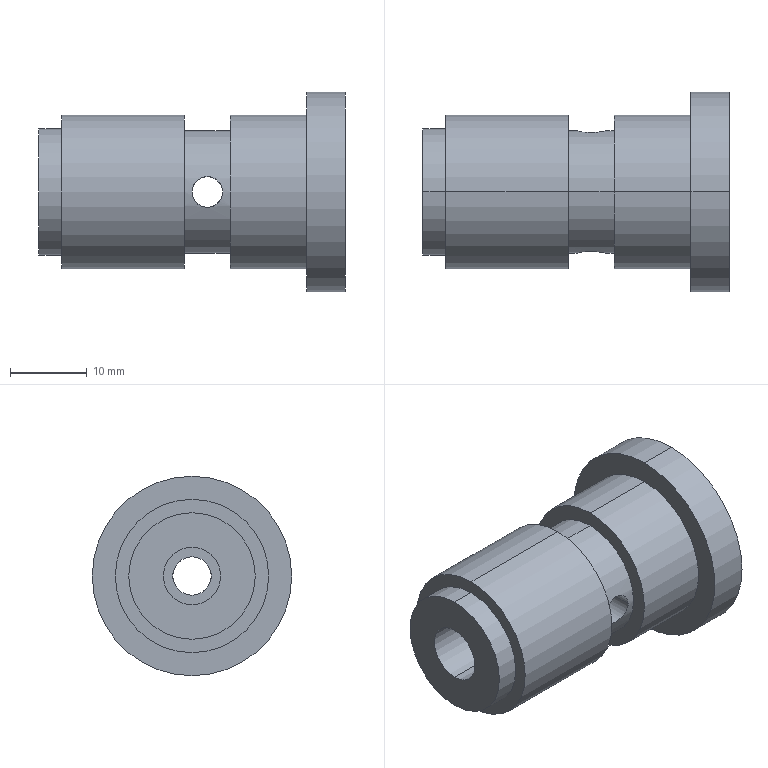Part | SolidWorks | features ICE 5, Cut 1, Extrusion 1, RevCut 1, SweepCut 1 | 1 solid | 34 faces | box 40 x 26 x 26 mm | volume 9972 mm3 | cylinder 24 | plane 10 | commonest cylinder face diameters 4 x4 16 x4 20 x4 5 x2 7.5 x2 14 x2
STEP:
#1=CARTESIAN_POINT('',(38.5,0.,-8.));
#2=VERTEX_POINT('',#1);
#3=CARTESIAN_POINT('',(38.5,0.,8.));
#4=VERTEX_POINT('',#3);
#5=CARTESIAN_POINT('',(38.5,0.,0.));
#6=DIRECTION('',(1.,0.,0.));
#7=DIRECTION('',(0.,0.,-1.));
#8=AXIS2_PLACEMENT_3D('',#5,#6,#7);
#9=CIRCLE('',#8,8.);
#10=EDGE_CURVE('',#2,#4,#9,.T.);
#11=ORIENTED_EDGE('',*,*,#10,.T.);
#12=CARTESIAN_POINT('',(40.,0.,8.));
#13=VERTEX_POINT('',#12);
#14=CARTESIAN_POINT('',(38.5,0.,8.));
#15=DIRECTION('',(1.,0.,0.));
#16=VECTOR('',#15,1000.);
#17=LINE('',#14,#16);
#18=EDGE_CURVE('',#4,#13,#17,.T.);
#19=ORIENTED_EDGE('',*,*,#18,.T.);
#20=CARTESIAN_POINT('',(40.,0.,-8.));
#21=VERTEX_POINT('',#20);
#22=CARTESIAN_POINT('',(40.,0.,0.));
#23=DIRECTION('',(1.,0.,0.));
#24=DIRECTION('',(0.,0.,-1.));
#25=AXIS2_PLACEMENT_3D('',#22,#23,#24);
#26=CIRCLE('',#25,8.);
#27=EDGE_CURVE('',#21,#13,#26,.T.);
#28=ORIENTED_EDGE('',*,*,#27,.F.);
#29=CARTESIAN_POINT('',(38.5,0.,-8.));
#30=DIRECTION('',(1.,0.,0.));
#31=VECTOR('',#30,1000.);
#32=LINE('',#29,#31);
#33=EDGE_CURVE('',#2,#21,#32,.T.);
#34=ORIENTED_EDGE('',*,*,#33,.F.);
#35=EDGE_LOOP('',(#11,#19,#28,#34));
#36=FACE_OUTER_BOUND('',#35,.T.);
#37=CARTESIAN_POINT('',(38.5,0.,0.));
#38=DIRECTION('',(1.,0.,0.));
#39=DIRECTION('',(0.,0.,-1.));
#40=AXIS2_PLACEMENT_3D('',#37,#38,#39);
#41=CYLINDRICAL_SURFACE('',#40,8.);
#42=ADVANCED_FACE('',(#36),#41,.T.);
#43=CARTESIAN_POINT('',(38.5,0.,11.));
#44=VERTEX_POINT('',#43);
#45=CARTESIAN_POINT('',(38.5,0.,-11.));
#46=VERTEX_POINT('',#45);
#47=CARTESIAN_POINT('',(38.5,0.,0.));
#48=DIRECTION('',(1.,0.,0.));
#49=DIRECTION('',(0.,0.,-1.));
#50=AXIS2_PLACEMENT_3D('',#47,#48,#49);
#51=CIRCLE('',#50,11.);
#52=EDGE_CURVE('',#44,#46,#51,.T.);
#53=ORIENTED_EDGE('',*,*,#52,.F.);
#54=CARTESIAN_POINT('',(40.,0.,11.));
#55=VERTEX_POINT('',#54);
#56=CARTESIAN_POINT('',(38.5,0.,11.));
#57=DIRECTION('',(1.,0.,0.));
#58=VECTOR('',#57,1000.);
#59=LINE('',#56,#58);
#60=EDGE_CURVE('',#44,#55,#59,.T.);
#61=ORIENTED_EDGE('',*,*,#60,.T.);
#62=CARTESIAN_POINT('',(40.,0.,-11.));
#63=VERTEX_POINT('',#62);
#64=CARTESIAN_POINT('',(40.,0.,0.));
#65=DIRECTION('',(1.,0.,0.));
#66=DIRECTION('',(0.,0.,-1.));
#67=AXIS2_PLACEMENT_3D('',#64,#65,#66);
#68=CIRCLE('',#67,11.);
#69=EDGE_CURVE('',#55,#63,#68,.T.);
#70=ORIENTED_EDGE('',*,*,#69,.T.);
#71=CARTESIAN_POINT('',(38.5,0.,-11.));
#72=DIRECTION('',(1.,0.,0.));
#73=VECTOR('',#72,1000.);
#74=LINE('',#71,#73);
#75=EDGE_CURVE('',#46,#63,#74,.T.);
#76=ORIENTED_EDGE('',*,*,#75,.F.);
#77=EDGE_LOOP('',(#53,#61,#70,#76));
#78=FACE_OUTER_BOUND('',#77,.T.);
#79=CARTESIAN_POINT('',(38.5,0.,0.));
#80=DIRECTION('',(1.,0.,0.));
#81=DIRECTION('',(0.,0.,-1.));
#82=AXIS2_PLACEMENT_3D('',#79,#80,#81);
#83=CYLINDRICAL_SURFACE('',#82,11.);
#84=ADVANCED_FACE('',(#78),#83,.F.);
#85=CARTESIAN_POINT('',(24.,8.,0.));
#86=VERTEX_POINT('',#85);
#87=CARTESIAN_POINT('',(20.,8.,0.));
#88=VERTEX_POINT('',#87);
#89=CARTESIAN_POINT('',(24.,8.,0.));
#90=CARTESIAN_POINT('',(24.,8.,-0.1327));
#91=CARTESIAN_POINT('',(23.987,7.997,-0.2631));
#92=CARTESIAN_POINT('',(23.936,7.984,-0.5195));
#93=CARTESIAN_POINT('',(23.897,7.975,-0.6468));
#94=CARTESIAN_POINT('',(23.796,7.951,-0.8888));
#95=CARTESIAN_POINT('',(23.735,7.938,-1.003));
#96=CARTESIAN_POINT('',(23.59,7.907,-1.22));
#97=CARTESIAN_POINT('',(23.506,7.89,-1.323));
#98=CARTESIAN_POINT('',(23.23,7.841,-1.598));
#99=CARTESIAN_POINT('',(23.008,7.808,-1.747));
#100=CARTESIAN_POINT('',(22.647,7.772,-1.897));
#101=CARTESIAN_POINT('',(22.52,7.762,-1.936));
#102=CARTESIAN_POINT('',(22.262,7.749,-1.987));
#103=CARTESIAN_POINT('',(22.132,7.746,-2.));
#104=CARTESIAN_POINT('',(21.87,7.746,-2.));
#105=CARTESIAN_POINT('',(21.737,7.749,-1.987));
#106=CARTESIAN_POINT('',(21.48,7.762,-1.936));
#107=CARTESIAN_POINT('',(21.355,7.772,-1.898));
#108=CARTESIAN_POINT('',(20.991,7.808,-1.746));
#109=CARTESIAN_POINT('',(20.771,7.841,-1.599));
#110=CARTESIAN_POINT('',(20.493,7.891,-1.321));
#111=CARTESIAN_POINT('',(20.41,7.907,-1.221));
#112=CARTESIAN_POINT('',(20.266,7.937,-1.005));
#113=CARTESIAN_POINT('',(20.203,7.952,-0.8874));
#114=CARTESIAN_POINT('',(20.103,7.975,-0.646));
#115=CARTESIAN_POINT('',(20.065,7.984,-0.5212));
#116=CARTESIAN_POINT('',(20.013,7.997,-0.2636));
#117=CARTESIAN_POINT('',(20.,8.,-0.1308));
#118=CARTESIAN_POINT('',(20.,8.,0.));
#119=B_SPLINE_CURVE_WITH_KNOTS('',3,(#89,#90,#91,#92,#93,#94,#95,#96,#97,#98,#99,#100,#101,#102,#103,#104,#105,#106,#107,#108,#109,#110,#111,#112,#113,#114,#115,#116,#117,#118),.UNSPECIFIED.,.F.,.F.,(4,2,2,2,2,2,2,2,2,2,2,2,2,2,4),(0.,0.0003924,0.0007847,0.001177,0.001569,0.002354,0.002747,0.003139,0.003531,0.003924,0.004708,0.005101,0.005493,0.005886,0.006278),.UNSPECIFIED.);
#120=EDGE_CURVE('',#86,#88,#119,.T.);
#121=ORIENTED_EDGE('',*,*,#120,.F.);
#122=CARTESIAN_POINT('',(20.,8.,0.));
#123=CARTESIAN_POINT('',(20.,8.,0.2616));
#124=CARTESIAN_POINT('',(20.053,7.986,0.5257));
#125=CARTESIAN_POINT('',(20.203,7.952,0.8871));
#126=CARTESIAN_POINT('',(20.265,7.937,1.004));
#127=CARTESIAN_POINT('',(20.411,7.907,1.221));
#128=CARTESIAN_POINT('',(20.493,7.891,1.321));
#129=CARTESIAN_POINT('',(20.677,7.858,1.506));
#130=CARTESIAN_POINT('',(20.78,7.841,1.59));
#131=CARTESIAN_POINT('',(20.996,7.81,1.734));
#132=CARTESIAN_POINT('',(21.11,7.796,1.796));
#133=CARTESIAN_POINT('',(21.475,7.76,1.948));
#134=CARTESIAN_POINT('',(21.736,7.746,2.));
#135=CARTESIAN_POINT('',(22.131,7.746,2.));
#136=CARTESIAN_POINT('',(22.261,7.749,1.987));
#137=CARTESIAN_POINT('',(22.518,7.762,1.936));
#138=CARTESIAN_POINT('',(22.646,7.772,1.897));
#139=CARTESIAN_POINT('',(23.008,7.808,1.747));
#140=CARTESIAN_POINT('',(23.23,7.841,1.598));
#141=CARTESIAN_POINT('',(23.597,7.907,1.232));
#142=CARTESIAN_POINT('',(23.746,7.94,1.01));
#143=CARTESIAN_POINT('',(23.896,7.975,0.6486));
#144=CARTESIAN_POINT('',(23.935,7.984,0.5212));
#145=CARTESIAN_POINT('',(23.987,7.997,0.2634));
#146=CARTESIAN_POINT('',(24.,8.,0.1327));
#147=CARTESIAN_POINT('',(24.,8.,0.));
#148=B_SPLINE_CURVE_WITH_KNOTS('',3,(#122,#123,#124,#125,#126,#127,#128,#129,#130,#131,#132,#133,#134,#135,#136,#137,#138,#139,#140,#141,#142,#143,#144,#145,#146,#147),.UNSPECIFIED.,.F.,.F.,(4,2,2,2,2,2,2,2,2,2,2,2,4),(0.006278,0.007062,0.007455,0.007847,0.008239,0.008631,0.009416,0.009808,0.0102,0.01099,0.01177,0.01216,0.01255),.UNSPECIFIED.);
#149=EDGE_CURVE('',#88,#86,#148,.T.);
#150=ORIENTED_EDGE('',*,*,#149,.F.);
#151=EDGE_LOOP('',(#121,#150));
#152=FACE_BOUND('',#151,.T.);
#153=CARTESIAN_POINT('',(19.,0.,-8.));
#154=VERTEX_POINT('',#153);
#155=CARTESIAN_POINT('',(19.,0.,8.));
#156=VERTEX_POINT('',#155);
#157=CARTESIAN_POINT('',(19.,0.,0.));
#158=DIRECTION('',(1.,0.,0.));
#159=DIRECTION('',(0.,0.,-1.));
#160=AXIS2_PLACEMENT_3D('',#157,#158,#159);
#161=CIRCLE('',#160,8.);
#162=EDGE_CURVE('',#154,#156,#161,.T.);
#163=ORIENTED_EDGE('',*,*,#162,.T.);
#164=CARTESIAN_POINT('',(25.,0.,8.));
#165=VERTEX_POINT('',#164);
#166=CARTESIAN_POINT('',(0.,0.,8.));
#167=DIRECTION('',(1.,0.,0.));
#168=VECTOR('',#167,1000.);
#169=LINE('',#166,#168);
#170=EDGE_CURVE('',#156,#165,#169,.T.);
#171=ORIENTED_EDGE('',*,*,#170,.T.);
#172=CARTESIAN_POINT('',(25.,0.,-8.));
#173=VERTEX_POINT('',#172);
#174=CARTESIAN_POINT('',(25.,0.,0.));
#175=DIRECTION('',(1.,0.,0.));
#176=DIRECTION('',(0.,0.,-1.));
#177=AXIS2_PLACEMENT_3D('',#174,#175,#176);
#178=CIRCLE('',#177,8.);
#179=EDGE_CURVE('',#173,#165,#178,.T.);
#180=ORIENTED_EDGE('',*,*,#179,.F.);
#181=CARTESIAN_POINT('',(0.,0.,-8.));
#182=DIRECTION('',(1.,0.,0.));
#183=VECTOR('',#182,1000.);
#184=LINE('',#181,#183);
#185=EDGE_CURVE('',#154,#173,#184,.T.);
#186=ORIENTED_EDGE('',*,*,#185,.F.);
#187=EDGE_LOOP('',(#163,#171,#180,#186));
#188=FACE_OUTER_BOUND('',#187,.T.);
#189=CARTESIAN_POINT('',(0.,0.,0.));
#190=DIRECTION('',(1.,0.,0.));
#191=DIRECTION('',(0.,0.,-1.));
#192=AXIS2_PLACEMENT_3D('',#189,#190,#191);
#193=CYLINDRICAL_SURFACE('',#192,8.);
#194=ADVANCED_FACE('',(#152,#188),#193,.T.);
#195=ORIENTED_EDGE('',*,*,#120,.T.);
#196=CARTESIAN_POINT('',(20.,2.5,0.));
#197=VERTEX_POINT('',#196);
#198=CARTESIAN_POINT('',(20.,11.268,0.));
#199=DIRECTION('',(0.,-1.,0.));
#200=VECTOR('',#199,1000.);
#201=LINE('',#198,#200);
#202=EDGE_CURVE('',#88,#197,#201,.T.);
#203=ORIENTED_EDGE('',*,*,#202,.T.);
#204=CARTESIAN_POINT('',(24.,2.5,0.));
#205=VERTEX_POINT('',#204);
#206=CARTESIAN_POINT('',(24.,2.5,0.));
#207=CARTESIAN_POINT('',(24.,2.5,-0.1403));
#208=CARTESIAN_POINT('',(23.985,2.488,-0.2771));
#209=CARTESIAN_POINT('',(23.929,2.444,-0.5445));
#210=CARTESIAN_POINT('',(23.887,2.41,-0.6754));
#211=CARTESIAN_POINT('',(23.782,2.329,-0.918));
#212=CARTESIAN_POINT('',(23.717,2.28,-1.033));
#213=CARTESIAN_POINT('',(23.572,2.172,-1.243));
#214=CARTESIAN_POINT('',(23.491,2.114,-1.339));
#215=CARTESIAN_POINT('',(23.314,1.993,-1.513));
#216=CARTESIAN_POINT('',(23.217,1.93,-1.592));
#217=CARTESIAN_POINT('',(23.01,1.807,-1.73));
#218=CARTESIAN_POINT('',(22.901,1.747,-1.79));
#219=CARTESIAN_POINT('',(22.668,1.639,-1.89));
#220=CARTESIAN_POINT('',(22.541,1.59,-1.93));
#221=CARTESIAN_POINT('',(22.278,1.52,-1.985));
#222=CARTESIAN_POINT('',(22.138,1.5,-2.));
#223=CARTESIAN_POINT('',(21.861,1.5,-2.));
#224=CARTESIAN_POINT('',(21.722,1.52,-1.985));
#225=CARTESIAN_POINT('',(21.458,1.59,-1.93));
#226=CARTESIAN_POINT('',(21.334,1.638,-1.89));
#227=CARTESIAN_POINT('',(20.979,1.802,-1.739));
#228=CARTESIAN_POINT('',(20.775,1.932,-1.601));
#229=CARTESIAN_POINT('',(20.508,2.115,-1.338));
#230=CARTESIAN_POINT('',(20.427,2.173,-1.242));
#231=CARTESIAN_POINT('',(20.283,2.279,-1.033));
#232=CARTESIAN_POINT('',(20.219,2.329,-0.9188));
#233=CARTESIAN_POINT('',(20.113,2.411,-0.6746));
#234=CARTESIAN_POINT('',(20.071,2.443,-0.5466));
#235=CARTESIAN_POINT('',(20.015,2.488,-0.2773));
#236=CARTESIAN_POINT('',(20.,2.5,-0.1381));
#237=CARTESIAN_POINT('',(20.,2.5,0.));
#238=B_SPLINE_CURVE_WITH_KNOTS('',3,(#206,#207,#208,#209,#210,#211,#212,#213,#214,#215,#216,#217,#218,#219,#220,#221,#222,#223,#224,#225,#226,#227,#228,#229,#230,#231,#232,#233,#234,#235,#236,#237),.UNSPECIFIED.,.F.,.F.,(4,2,2,2,2,2,2,2,2,2,2,2,2,2,2,4),(0.,0.0004139,0.0008279,0.001242,0.001656,0.00207,0.002484,0.002898,0.003311,0.003725,0.004139,0.004967,0.005381,0.005795,0.006209,0.006623),.UNSPECIFIED.);
#239=EDGE_CURVE('',#205,#197,#238,.T.);
#240=ORIENTED_EDGE('',*,*,#239,.F.);
#241=CARTESIAN_POINT('',(24.,11.268,0.));
#242=DIRECTION('',(0.,-1.,0.));
#243=VECTOR('',#242,1000.);
#244=LINE('',#241,#243);
#245=EDGE_CURVE('',#86,#205,#244,.T.);
#246=ORIENTED_EDGE('',*,*,#245,.F.);
#247=EDGE_LOOP('',(#195,#203,#240,#246));
#248=FACE_OUTER_BOUND('',#247,.T.);
#249=CARTESIAN_POINT('',(22.,11.268,0.));
#250=DIRECTION('',(0.,-1.,0.));
#251=DIRECTION('',(1.,0.,0.));
#252=AXIS2_PLACEMENT_3D('',#249,#250,#251);
#253=CYLINDRICAL_SURFACE('',#252,2.);
#254=ADVANCED_FACE('',(#248),#253,.F.);
#255=CARTESIAN_POINT('',(20.,-2.5,0.));
#256=VERTEX_POINT('',#255);
#257=CARTESIAN_POINT('',(24.,-2.5,0.));
#258=VERTEX_POINT('',#257);
#259=CARTESIAN_POINT('',(20.,-2.5,0.));
#260=CARTESIAN_POINT('',(20.,-2.5,-0.1377));
#261=CARTESIAN_POINT('',(20.015,-2.488,-0.2778));
#262=CARTESIAN_POINT('',(20.071,-2.444,-0.545));
#263=CARTESIAN_POINT('',(20.112,-2.411,-0.6743));
#264=CARTESIAN_POINT('',(20.271,-2.288,-1.04));
#265=CARTESIAN_POINT('',(20.421,-2.174,-1.252));
#266=CARTESIAN_POINT('',(20.775,-1.932,-1.6));
#267=CARTESIAN_POINT('',(20.982,-1.801,-1.74));
#268=CARTESIAN_POINT('',(21.331,-1.639,-1.889));
#269=CARTESIAN_POINT('',(21.456,-1.59,-1.929));
#270=CARTESIAN_POINT('',(21.72,-1.521,-1.985));
#271=CARTESIAN_POINT('',(21.859,-1.5,-2.));
#272=CARTESIAN_POINT('',(22.138,-1.5,-2.));
#273=CARTESIAN_POINT('',(22.276,-1.52,-1.986));
#274=CARTESIAN_POINT('',(22.541,-1.589,-1.93));
#275=CARTESIAN_POINT('',(22.664,-1.637,-1.891));
#276=CARTESIAN_POINT('',(22.9,-1.746,-1.791));
#277=CARTESIAN_POINT('',(23.011,-1.807,-1.73));
#278=CARTESIAN_POINT('',(23.216,-1.929,-1.593));
#279=CARTESIAN_POINT('',(23.312,-1.992,-1.515));
#280=CARTESIAN_POINT('',(23.49,-2.114,-1.34));
#281=CARTESIAN_POINT('',(23.572,-2.172,-1.243));
#282=CARTESIAN_POINT('',(23.716,-2.279,-1.034));
#283=CARTESIAN_POINT('',(23.78,-2.327,-0.9222));
#284=CARTESIAN_POINT('',(23.886,-2.41,-0.6783));
#285=CARTESIAN_POINT('',(23.928,-2.443,-0.5484));
#286=CARTESIAN_POINT('',(23.985,-2.488,-0.2808));
#287=CARTESIAN_POINT('',(24.,-2.5,-0.1398));
#288=CARTESIAN_POINT('',(24.,-2.5,0.));
#289=B_SPLINE_CURVE_WITH_KNOTS('',3,(#259,#260,#261,#262,#263,#264,#265,#266,#267,#268,#269,#270,#271,#272,#273,#274,#275,#276,#277,#278,#279,#280,#281,#282,#283,#284,#285,#286,#287,#288),.UNSPECIFIED.,.F.,.F.,(4,2,2,2,2,2,2,2,2,2,2,2,2,2,4),(0.006623,0.007035,0.007448,0.008273,0.009098,0.009511,0.009924,0.01034,0.01075,0.01116,0.01157,0.01199,0.0124,0.01281,0.01322),.UNSPECIFIED.);
#290=EDGE_CURVE('',#256,#258,#289,.T.);
#291=ORIENTED_EDGE('',*,*,#290,.F.);
#292=CARTESIAN_POINT('',(20.,-8.,0.));
#293=VERTEX_POINT('',#292);
#294=CARTESIAN_POINT('',(20.,11.268,0.));
#295=DIRECTION('',(0.,-1.,0.));
#296=VECTOR('',#295,1000.);
#297=LINE('',#294,#296);
#298=EDGE_CURVE('',#256,#293,#297,.T.);
#299=ORIENTED_EDGE('',*,*,#298,.T.);
#300=CARTESIAN_POINT('',(24.,-8.,0.));
#301=VERTEX_POINT('',#300);
#302=CARTESIAN_POINT('',(20.,-8.,0.));
#303=CARTESIAN_POINT('',(20.,-8.,-0.2616));
#304=CARTESIAN_POINT('',(20.053,-7.986,-0.5257));
#305=CARTESIAN_POINT('',(20.203,-7.952,-0.8871));
#306=CARTESIAN_POINT('',(20.265,-7.937,-1.004));
#307=CARTESIAN_POINT('',(20.411,-7.907,-1.221));
#308=CARTESIAN_POINT('',(20.493,-7.891,-1.321));
#309=CARTESIAN_POINT('',(20.677,-7.858,-1.506));
#310=CARTESIAN_POINT('',(20.78,-7.841,-1.59));
#311=CARTESIAN_POINT('',(20.996,-7.81,-1.734));
#312=CARTESIAN_POINT('',(21.11,-7.796,-1.796));
#313=CARTESIAN_POINT('',(21.475,-7.76,-1.948));
#314=CARTESIAN_POINT('',(21.736,-7.746,-2.));
#315=CARTESIAN_POINT('',(22.131,-7.746,-2.));
#316=CARTESIAN_POINT('',(22.261,-7.749,-1.987));
#317=CARTESIAN_POINT('',(22.518,-7.762,-1.936));
#318=CARTESIAN_POINT('',(22.646,-7.772,-1.897));
#319=CARTESIAN_POINT('',(23.008,-7.808,-1.747));
#320=CARTESIAN_POINT('',(23.23,-7.841,-1.598));
#321=CARTESIAN_POINT('',(23.597,-7.907,-1.232));
#322=CARTESIAN_POINT('',(23.746,-7.94,-1.01));
#323=CARTESIAN_POINT('',(23.896,-7.975,-0.6486));
#324=CARTESIAN_POINT('',(23.935,-7.984,-0.5212));
#325=CARTESIAN_POINT('',(23.987,-7.997,-0.2634));
#326=CARTESIAN_POINT('',(24.,-8.,-0.1327));
#327=CARTESIAN_POINT('',(24.,-8.,0.));
#328=B_SPLINE_CURVE_WITH_KNOTS('',3,(#302,#303,#304,#305,#306,#307,#308,#309,#310,#311,#312,#313,#314,#315,#316,#317,#318,#319,#320,#321,#322,#323,#324,#325,#326,#327),.UNSPECIFIED.,.F.,.F.,(4,2,2,2,2,2,2,2,2,2,2,2,4),(0.006278,0.007062,0.007455,0.007847,0.008239,0.008631,0.009416,0.009808,0.0102,0.01099,0.01177,0.01216,0.01255),.UNSPECIFIED.);
#329=EDGE_CURVE('',#293,#301,#328,.T.);
#330=ORIENTED_EDGE('',*,*,#329,.T.);
#331=CARTESIAN_POINT('',(24.,11.268,0.));
#332=DIRECTION('',(0.,-1.,0.));
#333=VECTOR('',#332,1000.);
#334=LINE('',#331,#333);
#335=EDGE_CURVE('',#258,#301,#334,.T.);
#336=ORIENTED_EDGE('',*,*,#335,.F.);
#337=EDGE_LOOP('',(#291,#299,#330,#336));
#338=FACE_OUTER_BOUND('',#337,.T.);
#339=CARTESIAN_POINT('',(22.,11.268,0.));
#340=DIRECTION('',(0.,-1.,0.));
#341=DIRECTION('',(1.,0.,0.));
#342=AXIS2_PLACEMENT_3D('',#339,#340,#341);
#343=CYLINDRICAL_SURFACE('',#342,2.);
#344=ADVANCED_FACE('',(#338),#343,.F.);
#345=CARTESIAN_POINT('',(6.5,0.,-3.75));
#346=VERTEX_POINT('',#345);
#347=CARTESIAN_POINT('',(6.5,0.,3.75));
#348=VERTEX_POINT('',#347);
#349=CARTESIAN_POINT('',(6.5,0.,0.));
#350=DIRECTION('',(-1.,0.,0.));
#351=DIRECTION('',(0.,0.,1.));
#352=AXIS2_PLACEMENT_3D('',#349,#350,#351);
#353=CIRCLE('',#352,3.75);
#354=EDGE_CURVE('',#346,#348,#353,.T.);
#355=ORIENTED_EDGE('',*,*,#354,.F.);
#356=CARTESIAN_POINT('',(0.,0.,-3.75));
#357=VERTEX_POINT('',#356);
#358=CARTESIAN_POINT('',(6.5,0.,-3.75));
#359=DIRECTION('',(-1.,0.,0.));
#360=VECTOR('',#359,1000.);
#361=LINE('',#358,#360);
#362=EDGE_CURVE('',#346,#357,#361,.T.);
#363=ORIENTED_EDGE('',*,*,#362,.T.);
#364=CARTESIAN_POINT('',(0.,0.,3.75));
#365=VERTEX_POINT('',#364);
#366=CARTESIAN_POINT('',(0.,0.,0.));
#367=DIRECTION('',(-1.,0.,0.));
#368=DIRECTION('',(0.,0.,1.));
#369=AXIS2_PLACEMENT_3D('',#366,#367,#368);
#370=CIRCLE('',#369,3.75);
#371=EDGE_CURVE('',#357,#365,#370,.T.);
#372=ORIENTED_EDGE('',*,*,#371,.T.);
#373=CARTESIAN_POINT('',(6.5,0.,3.75));
#374=DIRECTION('',(-1.,0.,0.));
#375=VECTOR('',#374,1000.);
#376=LINE('',#373,#375);
#377=EDGE_CURVE('',#348,#365,#376,.T.);
#378=ORIENTED_EDGE('',*,*,#377,.F.);
#379=EDGE_LOOP('',(#355,#363,#372,#378));
#380=FACE_OUTER_BOUND('',#379,.T.);
#381=CARTESIAN_POINT('',(6.5,0.,0.));
#382=DIRECTION('',(-1.,0.,0.));
#383=DIRECTION('',(0.,0.,1.));
#384=AXIS2_PLACEMENT_3D('',#381,#382,#383);
#385=CYLINDRICAL_SURFACE('',#384,3.75);
#386=ADVANCED_FACE('',(#380),#385,.F.);
#387=CARTESIAN_POINT('',(30.,0.,7.));
#388=VERTEX_POINT('',#387);
#389=CARTESIAN_POINT('',(30.,0.,-7.));
#390=VERTEX_POINT('',#389);
#391=CARTESIAN_POINT('',(30.,0.,0.));
#392=DIRECTION('',(1.,0.,0.));
#393=DIRECTION('',(0.,0.,-1.));
#394=AXIS2_PLACEMENT_3D('',#391,#392,#393);
#395=CIRCLE('',#394,7.);
#396=EDGE_CURVE('',#388,#390,#395,.T.);
#397=ORIENTED_EDGE('',*,*,#396,.F.);
#398=CARTESIAN_POINT('',(40.,0.,7.));
#399=VERTEX_POINT('',#398);
#400=CARTESIAN_POINT('',(30.,0.,7.));
#401=DIRECTION('',(1.,0.,0.));
#402=VECTOR('',#401,1000.);
#403=LINE('',#400,#402);
#404=EDGE_CURVE('',#388,#399,#403,.T.);
#405=ORIENTED_EDGE('',*,*,#404,.T.);
#406=CARTESIAN_POINT('',(40.,0.,-7.));
#407=VERTEX_POINT('',#406);
#408=CARTESIAN_POINT('',(40.,0.,0.));
#409=DIRECTION('',(1.,0.,0.));
#410=DIRECTION('',(0.,0.,-1.));
#411=AXIS2_PLACEMENT_3D('',#408,#409,#410);
#412=CIRCLE('',#411,7.);
#413=EDGE_CURVE('',#399,#407,#412,.T.);
#414=ORIENTED_EDGE('',*,*,#413,.T.);
#415=CARTESIAN_POINT('',(30.,0.,-7.));
#416=DIRECTION('',(1.,0.,0.));
#417=VECTOR('',#416,1000.);
#418=LINE('',#415,#417);
#419=EDGE_CURVE('',#390,#407,#418,.T.);
#420=ORIENTED_EDGE('',*,*,#419,.F.);
#421=EDGE_LOOP('',(#397,#405,#414,#420));
#422=FACE_OUTER_BOUND('',#421,.T.);
#423=CARTESIAN_POINT('',(30.,0.,0.));
#424=DIRECTION('',(1.,0.,0.));
#425=DIRECTION('',(0.,0.,-1.));
#426=AXIS2_PLACEMENT_3D('',#423,#424,#425);
#427=CYLINDRICAL_SURFACE('',#426,7.);
#428=ADVANCED_FACE('',(#422),#427,.F.);
#429=CARTESIAN_POINT('',(40.,0.,-13.));
#430=VERTEX_POINT('',#429);
#431=CARTESIAN_POINT('',(40.,0.,13.));
#432=VERTEX_POINT('',#431);
#433=CARTESIAN_POINT('',(40.,0.,0.));
#434=DIRECTION('',(1.,0.,0.));
#435=DIRECTION('',(0.,0.,-1.));
#436=AXIS2_PLACEMENT_3D('',#433,#434,#435);
#437=CIRCLE('',#436,13.);
#438=EDGE_CURVE('',#430,#432,#437,.T.);
#439=ORIENTED_EDGE('',*,*,#438,.F.);
#440=CARTESIAN_POINT('',(35.,0.,-13.));
#441=VERTEX_POINT('',#440);
#442=CARTESIAN_POINT('',(40.,0.,-13.));
#443=DIRECTION('',(-1.,0.,0.));
#444=VECTOR('',#443,1000.);
#445=LINE('',#442,#444);
#446=EDGE_CURVE('',#430,#441,#445,.T.);
#447=ORIENTED_EDGE('',*,*,#446,.T.);
#448=CARTESIAN_POINT('',(35.,0.,13.));
#449=VERTEX_POINT('',#448);
#450=CARTESIAN_POINT('',(35.,0.,0.));
#451=DIRECTION('',(1.,0.,0.));
#452=DIRECTION('',(0.,0.,-1.));
#453=AXIS2_PLACEMENT_3D('',#450,#451,#452);
#454=CIRCLE('',#453,13.);
#455=EDGE_CURVE('',#441,#449,#454,.T.);
#456=ORIENTED_EDGE('',*,*,#455,.T.);
#457=CARTESIAN_POINT('',(40.,0.,13.));
#458=DIRECTION('',(-1.,0.,0.));
#459=VECTOR('',#458,1000.);
#460=LINE('',#457,#459);
#461=EDGE_CURVE('',#432,#449,#460,.T.);
#462=ORIENTED_EDGE('',*,*,#461,.F.);
#463=EDGE_LOOP('',(#439,#447,#456,#462));
#464=FACE_OUTER_BOUND('',#463,.T.);
#465=CARTESIAN_POINT('',(40.,0.,0.));
#466=DIRECTION('',(-1.,0.,0.));
#467=DIRECTION('',(0.,0.,1.));
#468=AXIS2_PLACEMENT_3D('',#465,#466,#467);
#469=CYLINDRICAL_SURFACE('',#468,13.);
#470=ADVANCED_FACE('',(#464),#469,.T.);
#471=CARTESIAN_POINT('',(19.,0.,10.));
#472=VERTEX_POINT('',#471);
#473=CARTESIAN_POINT('',(19.,0.,-10.));
#474=VERTEX_POINT('',#473);
#475=CARTESIAN_POINT('',(19.,0.,0.));
#476=DIRECTION('',(-1.,0.,0.));
#477=DIRECTION('',(0.,0.,1.));
#478=AXIS2_PLACEMENT_3D('',#475,#476,#477);
#479=CIRCLE('',#478,10.);
#480=EDGE_CURVE('',#472,#474,#479,.T.);
#481=ORIENTED_EDGE('',*,*,#480,.T.);
#482=CARTESIAN_POINT('',(3.,0.,-10.));
#483=VERTEX_POINT('',#482);
#484=CARTESIAN_POINT('',(35.,0.,-10.));
#485=DIRECTION('',(-1.,0.,0.));
#486=VECTOR('',#485,1000.);
#487=LINE('',#484,#486);
#488=EDGE_CURVE('',#474,#483,#487,.T.);
#489=ORIENTED_EDGE('',*,*,#488,.T.);
#490=CARTESIAN_POINT('',(3.,0.,10.));
#491=VERTEX_POINT('',#490);
#492=CARTESIAN_POINT('',(3.,0.,0.));
#493=DIRECTION('',(1.,0.,0.));
#494=DIRECTION('',(0.,0.,-1.));
#495=AXIS2_PLACEMENT_3D('',#492,#493,#494);
#496=CIRCLE('',#495,10.);
#497=EDGE_CURVE('',#483,#491,#496,.T.);
#498=ORIENTED_EDGE('',*,*,#497,.T.);
#499=CARTESIAN_POINT('',(35.,0.,10.));
#500=DIRECTION('',(-1.,0.,0.));
#501=VECTOR('',#500,1000.);
#502=LINE('',#499,#501);
#503=EDGE_CURVE('',#472,#491,#502,.T.);
#504=ORIENTED_EDGE('',*,*,#503,.F.);
#505=EDGE_LOOP('',(#481,#489,#498,#504));
#506=FACE_OUTER_BOUND('',#505,.T.);
#507=CARTESIAN_POINT('',(35.,0.,0.));
#508=DIRECTION('',(-1.,0.,0.));
#509=DIRECTION('',(0.,0.,1.));
#510=AXIS2_PLACEMENT_3D('',#507,#508,#509);
#511=CYLINDRICAL_SURFACE('',#510,10.);
#512=ADVANCED_FACE('',(#506),#511,.T.);
#513=CARTESIAN_POINT('',(3.,0.,-8.25));
#514=VERTEX_POINT('',#513);
#515=CARTESIAN_POINT('',(3.,0.,8.25));
#516=VERTEX_POINT('',#515);
#517=CARTESIAN_POINT('',(3.,0.,0.));
#518=DIRECTION('',(1.,0.,0.));
#519=DIRECTION('',(0.,0.,-1.));
#520=AXIS2_PLACEMENT_3D('',#517,#518,#519);
#521=CIRCLE('',#520,8.25);
#522=EDGE_CURVE('',#514,#516,#521,.T.);
#523=ORIENTED_EDGE('',*,*,#522,.F.);
#524=CARTESIAN_POINT('',(0.,0.,-8.25));
#525=VERTEX_POINT('',#524);
#526=CARTESIAN_POINT('',(3.,0.,-8.25));
#527=DIRECTION('',(-1.,0.,0.));
#528=VECTOR('',#527,1000.);
#529=LINE('',#526,#528);
#530=EDGE_CURVE('',#514,#525,#529,.T.);
#531=ORIENTED_EDGE('',*,*,#530,.T.);
#532=CARTESIAN_POINT('',(0.,0.,8.25));
#533=VERTEX_POINT('',#532);
#534=CARTESIAN_POINT('',(0.,0.,0.));
#535=DIRECTION('',(1.,0.,0.));
#536=DIRECTION('',(0.,0.,-1.));
#537=AXIS2_PLACEMENT_3D('',#534,#535,#536);
#538=CIRCLE('',#537,8.25);
#539=EDGE_CURVE('',#525,#533,#538,.T.);
#540=ORIENTED_EDGE('',*,*,#539,.T.);
#541=CARTESIAN_POINT('',(3.,0.,8.25));
#542=DIRECTION('',(-1.,0.,0.));
#543=VECTOR('',#542,1000.);
#544=LINE('',#541,#543);
#545=EDGE_CURVE('',#516,#533,#544,.T.);
#546=ORIENTED_EDGE('',*,*,#545,.F.);
#547=EDGE_LOOP('',(#523,#531,#540,#546));
#548=FACE_OUTER_BOUND('',#547,.T.);
#549=CARTESIAN_POINT('',(3.,0.,0.));
#550=DIRECTION('',(-1.,0.,0.));
#551=DIRECTION('',(0.,0.,1.));
#552=AXIS2_PLACEMENT_3D('',#549,#550,#551);
#553=CYLINDRICAL_SURFACE('',#552,8.25);
#554=ADVANCED_FACE('',(#548),#553,.T.);
#555=CARTESIAN_POINT('',(24.,-2.5,0.));
#556=CARTESIAN_POINT('',(24.,-2.5,0.1403));
#557=CARTESIAN_POINT('',(23.985,-2.488,0.2771));
#558=CARTESIAN_POINT('',(23.929,-2.444,0.5445));
#559=CARTESIAN_POINT('',(23.887,-2.41,0.6754));
#560=CARTESIAN_POINT('',(23.782,-2.329,0.918));
#561=CARTESIAN_POINT('',(23.717,-2.28,1.033));
#562=CARTESIAN_POINT('',(23.572,-2.172,1.243));
#563=CARTESIAN_POINT('',(23.491,-2.114,1.339));
#564=CARTESIAN_POINT('',(23.314,-1.993,1.513));
#565=CARTESIAN_POINT('',(23.217,-1.93,1.592));
#566=CARTESIAN_POINT('',(23.01,-1.807,1.73));
#567=CARTESIAN_POINT('',(22.901,-1.747,1.79));
#568=CARTESIAN_POINT('',(22.668,-1.639,1.89));
#569=CARTESIAN_POINT('',(22.541,-1.59,1.93));
#570=CARTESIAN_POINT('',(22.278,-1.52,1.985));
#571=CARTESIAN_POINT('',(22.138,-1.5,2.));
#572=CARTESIAN_POINT('',(21.861,-1.5,2.));
#573=CARTESIAN_POINT('',(21.722,-1.52,1.985));
#574=CARTESIAN_POINT('',(21.458,-1.59,1.93));
#575=CARTESIAN_POINT('',(21.334,-1.638,1.89));
#576=CARTESIAN_POINT('',(20.979,-1.802,1.739));
#577=CARTESIAN_POINT('',(20.775,-1.932,1.601));
#578=CARTESIAN_POINT('',(20.508,-2.115,1.338));
#579=CARTESIAN_POINT('',(20.427,-2.173,1.242));
#580=CARTESIAN_POINT('',(20.283,-2.279,1.033));
#581=CARTESIAN_POINT('',(20.219,-2.329,0.9188));
#582=CARTESIAN_POINT('',(20.113,-2.411,0.6746));
#583=CARTESIAN_POINT('',(20.071,-2.443,0.5466));
#584=CARTESIAN_POINT('',(20.015,-2.488,0.2773));
#585=CARTESIAN_POINT('',(20.,-2.5,0.1381));
#586=CARTESIAN_POINT('',(20.,-2.5,0.));
#587=B_SPLINE_CURVE_WITH_KNOTS('',3,(#555,#556,#557,#558,#559,#560,#561,#562,#563,#564,#565,#566,#567,#568,#569,#570,#571,#572,#573,#574,#575,#576,#577,#578,#579,#580,#581,#582,#583,#584,#585,#586),.UNSPECIFIED.,.F.,.F.,(4,2,2,2,2,2,2,2,2,2,2,2,2,2,2,4),(0.,0.0004139,0.0008279,0.001242,0.001656,0.00207,0.002484,0.002898,0.003311,0.003725,0.004139,0.004967,0.005381,0.005795,0.006209,0.006623),.UNSPECIFIED.);
#588=EDGE_CURVE('',#258,#256,#587,.T.);
#589=ORIENTED_EDGE('',*,*,#588,.T.);
#590=ORIENTED_EDGE('',*,*,#290,.T.);
#591=EDGE_LOOP('',(#589,#590));
#592=FACE_BOUND('',#591,.T.);
#593=CARTESIAN_POINT('',(6.5,0.,2.5));
#594=VERTEX_POINT('',#593);
#595=CARTESIAN_POINT('',(6.5,0.,-2.5));
#596=VERTEX_POINT('',#595);
#597=CARTESIAN_POINT('',(6.5,0.,0.));
#598=DIRECTION('',(1.,0.,0.));
#599=DIRECTION('',(0.,0.,1.));
#600=AXIS2_PLACEMENT_3D('',#597,#598,#599);
#601=CIRCLE('',#600,2.5);
#602=EDGE_CURVE('',#594,#596,#601,.T.);
#603=ORIENTED_EDGE('',*,*,#602,.F.);
#604=CARTESIAN_POINT('',(30.,0.,2.5));
#605=VERTEX_POINT('',#604);
#606=CARTESIAN_POINT('',(-3.,0.,2.5));
#607=DIRECTION('',(1.,0.,0.));
#608=VECTOR('',#607,1000.);
#609=LINE('',#606,#608);
#610=EDGE_CURVE('',#594,#605,#609,.T.);
#611=ORIENTED_EDGE('',*,*,#610,.T.);
#612=CARTESIAN_POINT('',(30.,0.,-2.5));
#613=VERTEX_POINT('',#612);
#614=CARTESIAN_POINT('',(30.,0.,0.));
#615=DIRECTION('',(1.,0.,0.));
#616=DIRECTION('',(0.,0.,-1.));
#617=AXIS2_PLACEMENT_3D('',#614,#615,#616);
#618=CIRCLE('',#617,2.5);
#619=EDGE_CURVE('',#605,#613,#618,.T.);
#620=ORIENTED_EDGE('',*,*,#619,.T.);
#621=CARTESIAN_POINT('',(-3.,0.,-2.5));
#622=DIRECTION('',(1.,0.,0.));
#623=VECTOR('',#622,1000.);
#624=LINE('',#621,#623);
#625=EDGE_CURVE('',#596,#613,#624,.T.);
#626=ORIENTED_EDGE('',*,*,#625,.F.);
#627=EDGE_LOOP('',(#603,#611,#620,#626));
#628=FACE_OUTER_BOUND('',#627,.T.);
#629=CARTESIAN_POINT('',(-3.,0.,0.));
#630=DIRECTION('',(1.,0.,0.));
#631=DIRECTION('',(0.,0.,-1.));
#632=AXIS2_PLACEMENT_3D('',#629,#630,#631);
#633=CYLINDRICAL_SURFACE('',#632,2.5);
#634=ADVANCED_FACE('',(#592,#628),#633,.F.);
#635=CARTESIAN_POINT('',(35.,0.,-10.));
#636=VERTEX_POINT('',#635);
#637=CARTESIAN_POINT('',(35.,0.,10.));
#638=VERTEX_POINT('',#637);
#639=CARTESIAN_POINT('',(35.,0.,0.));
#640=DIRECTION('',(1.,0.,0.));
#641=DIRECTION('',(0.,0.,-1.));
#642=AXIS2_PLACEMENT_3D('',#639,#640,#641);
#643=CIRCLE('',#642,10.);
#644=EDGE_CURVE('',#636,#638,#643,.T.);
#645=ORIENTED_EDGE('',*,*,#644,.F.);
#646=CARTESIAN_POINT('',(25.,0.,-10.));
#647=VERTEX_POINT('',#646);
#648=CARTESIAN_POINT('',(35.,0.,-10.));
#649=DIRECTION('',(-1.,0.,0.));
#650=VECTOR('',#649,1000.);
#651=LINE('',#648,#650);
#652=EDGE_CURVE('',#636,#647,#651,.T.);
#653=ORIENTED_EDGE('',*,*,#652,.T.);
#654=CARTESIAN_POINT('',(25.,0.,10.));
#655=VERTEX_POINT('',#654);
#656=CARTESIAN_POINT('',(25.,0.,0.));
#657=DIRECTION('',(1.,0.,0.));
#658=DIRECTION('',(0.,0.,-1.));
#659=AXIS2_PLACEMENT_3D('',#656,#657,#658);
#660=CIRCLE('',#659,10.);
#661=EDGE_CURVE('',#647,#655,#660,.T.);
#662=ORIENTED_EDGE('',*,*,#661,.T.);
#663=CARTESIAN_POINT('',(35.,0.,10.));
#664=DIRECTION('',(-1.,0.,0.));
#665=VECTOR('',#664,1000.);
#666=LINE('',#663,#665);
#667=EDGE_CURVE('',#638,#655,#666,.T.);
#668=ORIENTED_EDGE('',*,*,#667,.F.);
#669=EDGE_LOOP('',(#645,#653,#662,#668));
#670=FACE_OUTER_BOUND('',#669,.T.);
#671=CARTESIAN_POINT('',(35.,0.,0.));
#672=DIRECTION('',(-1.,0.,0.));
#673=DIRECTION('',(0.,0.,1.));
#674=AXIS2_PLACEMENT_3D('',#671,#672,#673);
#675=CYLINDRICAL_SURFACE('',#674,10.);
#676=ADVANCED_FACE('',(#670),#675,.T.);
#677=CARTESIAN_POINT('',(40.,0.,0.));
#678=DIRECTION('',(1.,0.,0.));
#679=DIRECTION('',(0.,0.,-1.));
#680=AXIS2_PLACEMENT_3D('',#677,#678,#679);
#681=CIRCLE('',#680,7.);
#682=EDGE_CURVE('',#407,#399,#681,.T.);
#683=ORIENTED_EDGE('',*,*,#682,.F.);
#684=ORIENTED_EDGE('',*,*,#413,.F.);
#685=EDGE_LOOP('',(#683,#684));
#686=FACE_BOUND('',#685,.T.);
#687=ORIENTED_EDGE('',*,*,#27,.T.);
#688=CARTESIAN_POINT('',(40.,0.,0.));
#689=DIRECTION('',(1.,0.,0.));
#690=DIRECTION('',(0.,0.,-1.));
#691=AXIS2_PLACEMENT_3D('',#688,#689,#690);
#692=CIRCLE('',#691,8.);
#693=EDGE_CURVE('',#13,#21,#692,.T.);
#694=ORIENTED_EDGE('',*,*,#693,.T.);
#695=EDGE_LOOP('',(#687,#694));
#696=FACE_OUTER_BOUND('',#695,.T.);
#697=CARTESIAN_POINT('',(40.,0.,0.));
#698=DIRECTION('',(1.,0.,0.));
#699=DIRECTION('',(0.,0.,-1.));
#700=AXIS2_PLACEMENT_3D('',#697,#698,#699);
#701=PLANE('',#700);
#702=ADVANCED_FACE('',(#686,#696),#701,.T.);
#703=ORIENTED_EDGE('',*,*,#652,.F.);
#704=CARTESIAN_POINT('',(35.,0.,0.));
#705=DIRECTION('',(1.,0.,0.));
#706=DIRECTION('',(0.,0.,-1.));
#707=AXIS2_PLACEMENT_3D('',#704,#705,#706);
#708=CIRCLE('',#707,10.);
#709=EDGE_CURVE('',#638,#636,#708,.T.);
#710=ORIENTED_EDGE('',*,*,#709,.F.);
#711=ORIENTED_EDGE('',*,*,#667,.T.);
#712=CARTESIAN_POINT('',(25.,0.,0.));
#713=DIRECTION('',(1.,0.,0.));
#714=DIRECTION('',(0.,0.,-1.));
#715=AXIS2_PLACEMENT_3D('',#712,#713,#714);
#716=CIRCLE('',#715,10.);
#717=EDGE_CURVE('',#655,#647,#716,.T.);
#718=ORIENTED_EDGE('',*,*,#717,.T.);
#719=EDGE_LOOP('',(#703,#710,#711,#718));
#720=FACE_OUTER_BOUND('',#719,.T.);
#721=CARTESIAN_POINT('',(35.,0.,0.));
#722=DIRECTION('',(-1.,0.,0.));
#723=DIRECTION('',(0.,0.,1.));
#724=AXIS2_PLACEMENT_3D('',#721,#722,#723);
#725=CYLINDRICAL_SURFACE('',#724,10.);
#726=ADVANCED_FACE('',(#720),#725,.T.);
#727=ORIENTED_EDGE('',*,*,#610,.F.);
#728=CARTESIAN_POINT('',(6.5,0.,0.));
#729=DIRECTION('',(1.,0.,0.));
#730=DIRECTION('',(0.,0.,1.));
#731=AXIS2_PLACEMENT_3D('',#728,#729,#730);
#732=CIRCLE('',#731,2.5);
#733=EDGE_CURVE('',#596,#594,#732,.T.);
#734=ORIENTED_EDGE('',*,*,#733,.F.);
#735=ORIENTED_EDGE('',*,*,#625,.T.);
#736=CARTESIAN_POINT('',(30.,0.,0.));
#737=DIRECTION('',(1.,0.,0.));
#738=DIRECTION('',(0.,0.,-1.));
#739=AXIS2_PLACEMENT_3D('',#736,#737,#738);
#740=CIRCLE('',#739,2.5);
#741=EDGE_CURVE('',#613,#605,#740,.T.);
#742=ORIENTED_EDGE('',*,*,#741,.T.);
#743=EDGE_LOOP('',(#727,#734,#735,#742));
#744=FACE_OUTER_BOUND('',#743,.T.);
#745=ORIENTED_EDGE('',*,*,#239,.T.);
#746=CARTESIAN_POINT('',(20.,2.5,0.));
#747=CARTESIAN_POINT('',(20.,2.5,0.1377));
#748=CARTESIAN_POINT('',(20.015,2.488,0.2778));
#749=CARTESIAN_POINT('',(20.071,2.444,0.545));
#750=CARTESIAN_POINT('',(20.112,2.411,0.6743));
#751=CARTESIAN_POINT('',(20.271,2.288,1.04));
#752=CARTESIAN_POINT('',(20.421,2.174,1.252));
#753=CARTESIAN_POINT('',(20.775,1.932,1.6));
#754=CARTESIAN_POINT('',(20.982,1.801,1.74));
#755=CARTESIAN_POINT('',(21.331,1.639,1.889));
#756=CARTESIAN_POINT('',(21.456,1.59,1.929));
#757=CARTESIAN_POINT('',(21.72,1.521,1.985));
#758=CARTESIAN_POINT('',(21.859,1.5,2.));
#759=CARTESIAN_POINT('',(22.138,1.5,2.));
#760=CARTESIAN_POINT('',(22.276,1.52,1.986));
#761=CARTESIAN_POINT('',(22.541,1.589,1.93));
#762=CARTESIAN_POINT('',(22.664,1.637,1.891));
#763=CARTESIAN_POINT('',(22.9,1.746,1.791));
#764=CARTESIAN_POINT('',(23.011,1.807,1.73));
#765=CARTESIAN_POINT('',(23.216,1.929,1.593));
#766=CARTESIAN_POINT('',(23.312,1.992,1.515));
#767=CARTESIAN_POINT('',(23.49,2.114,1.34));
#768=CARTESIAN_POINT('',(23.572,2.172,1.243));
#769=CARTESIAN_POINT('',(23.716,2.279,1.034));
#770=CARTESIAN_POINT('',(23.78,2.327,0.9222));
#771=CARTESIAN_POINT('',(23.886,2.41,0.6783));
#772=CARTESIAN_POINT('',(23.928,2.443,0.5484));
#773=CARTESIAN_POINT('',(23.985,2.488,0.2808));
#774=CARTESIAN_POINT('',(24.,2.5,0.1398));
#775=CARTESIAN_POINT('',(24.,2.5,0.));
#776=B_SPLINE_CURVE_WITH_KNOTS('',3,(#746,#747,#748,#749,#750,#751,#752,#753,#754,#755,#756,#757,#758,#759,#760,#761,#762,#763,#764,#765,#766,#767,#768,#769,#770,#771,#772,#773,#774,#775),.UNSPECIFIED.,.F.,.F.,(4,2,2,2,2,2,2,2,2,2,2,2,2,2,4),(0.006623,0.007035,0.007448,0.008273,0.009098,0.009511,0.009924,0.01034,0.01075,0.01116,0.01157,0.01199,0.0124,0.01281,0.01322),.UNSPECIFIED.);
#777=EDGE_CURVE('',#197,#205,#776,.T.);
#778=ORIENTED_EDGE('',*,*,#777,.T.);
#779=EDGE_LOOP('',(#745,#778));
#780=FACE_BOUND('',#779,.T.);
#781=CARTESIAN_POINT('',(-3.,0.,0.));
#782=DIRECTION('',(1.,0.,0.));
#783=DIRECTION('',(0.,0.,-1.));
#784=AXIS2_PLACEMENT_3D('',#781,#782,#783);
#785=CYLINDRICAL_SURFACE('',#784,2.5);
#786=ADVANCED_FACE('',(#744,#780),#785,.F.);
#787=ORIENTED_EDGE('',*,*,#530,.F.);
#788=CARTESIAN_POINT('',(3.,0.,0.));
#789=DIRECTION('',(1.,0.,0.));
#790=DIRECTION('',(0.,0.,-1.));
#791=AXIS2_PLACEMENT_3D('',#788,#789,#790);
#792=CIRCLE('',#791,8.25);
#793=EDGE_CURVE('',#516,#514,#792,.T.);
#794=ORIENTED_EDGE('',*,*,#793,.F.);
#795=ORIENTED_EDGE('',*,*,#545,.T.);
#796=CARTESIAN_POINT('',(0.,0.,0.));
#797=DIRECTION('',(1.,0.,0.));
#798=DIRECTION('',(0.,0.,-1.));
#799=AXIS2_PLACEMENT_3D('',#796,#797,#798);
#800=CIRCLE('',#799,8.25);
#801=EDGE_CURVE('',#533,#525,#800,.T.);
#802=ORIENTED_EDGE('',*,*,#801,.T.);
#803=EDGE_LOOP('',(#787,#794,#795,#802));
#804=FACE_OUTER_BOUND('',#803,.T.);
#805=CARTESIAN_POINT('',(3.,0.,0.));
#806=DIRECTION('',(-1.,0.,0.));
#807=DIRECTION('',(0.,0.,1.));
#808=AXIS2_PLACEMENT_3D('',#805,#806,#807);
#809=CYLINDRICAL_SURFACE('',#808,8.25);
#810=ADVANCED_FACE('',(#804),#809,.T.);
#811=CARTESIAN_POINT('',(0.,0.,0.));
#812=DIRECTION('',(-1.,0.,0.));
#813=DIRECTION('',(0.,0.,1.));
#814=AXIS2_PLACEMENT_3D('',#811,#812,#813);
#815=CIRCLE('',#814,3.75);
#816=EDGE_CURVE('',#365,#357,#815,.T.);
#817=ORIENTED_EDGE('',*,*,#816,.F.);
#818=ORIENTED_EDGE('',*,*,#371,.F.);
#819=EDGE_LOOP('',(#817,#818));
#820=FACE_BOUND('',#819,.T.);
#821=ORIENTED_EDGE('',*,*,#801,.F.);
#822=ORIENTED_EDGE('',*,*,#539,.F.);
#823=EDGE_LOOP('',(#821,#822));
#824=FACE_OUTER_BOUND('',#823,.T.);
#825=CARTESIAN_POINT('',(0.,0.,0.));
#826=DIRECTION('',(1.,0.,0.));
#827=DIRECTION('',(0.,0.,-1.));
#828=AXIS2_PLACEMENT_3D('',#825,#826,#827);
#829=PLANE('',#828);
#830=ADVANCED_FACE('',(#820,#824),#829,.F.);
#831=ORIENTED_EDGE('',*,*,#488,.F.);
#832=CARTESIAN_POINT('',(19.,0.,0.));
#833=DIRECTION('',(-1.,0.,0.));
#834=DIRECTION('',(0.,0.,1.));
#835=AXIS2_PLACEMENT_3D('',#832,#833,#834);
#836=CIRCLE('',#835,10.);
#837=EDGE_CURVE('',#474,#472,#836,.T.);
#838=ORIENTED_EDGE('',*,*,#837,.T.);
#839=ORIENTED_EDGE('',*,*,#503,.T.);
#840=CARTESIAN_POINT('',(3.,0.,0.));
#841=DIRECTION('',(1.,0.,0.));
#842=DIRECTION('',(0.,0.,-1.));
#843=AXIS2_PLACEMENT_3D('',#840,#841,#842);
#844=CIRCLE('',#843,10.);
#845=EDGE_CURVE('',#491,#483,#844,.T.);
#846=ORIENTED_EDGE('',*,*,#845,.T.);
#847=EDGE_LOOP('',(#831,#838,#839,#846));
#848=FACE_OUTER_BOUND('',#847,.T.);
#849=CARTESIAN_POINT('',(35.,0.,0.));
#850=DIRECTION('',(-1.,0.,0.));
#851=DIRECTION('',(0.,0.,1.));
#852=AXIS2_PLACEMENT_3D('',#849,#850,#851);
#853=CYLINDRICAL_SURFACE('',#852,10.);
#854=ADVANCED_FACE('',(#848),#853,.T.);
#855=ORIENTED_EDGE('',*,*,#793,.T.);
#856=ORIENTED_EDGE('',*,*,#522,.T.);
#857=EDGE_LOOP('',(#855,#856));
#858=FACE_BOUND('',#857,.T.);
#859=ORIENTED_EDGE('',*,*,#845,.F.);
#860=ORIENTED_EDGE('',*,*,#497,.F.);
#861=EDGE_LOOP('',(#859,#860));
#862=FACE_OUTER_BOUND('',#861,.T.);
#863=CARTESIAN_POINT('',(3.,0.,0.));
#864=DIRECTION('',(1.,0.,0.));
#865=DIRECTION('',(0.,0.,-1.));
#866=AXIS2_PLACEMENT_3D('',#863,#864,#865);
#867=PLANE('',#866);
#868=ADVANCED_FACE('',(#858,#862),#867,.F.);
#869=ORIENTED_EDGE('',*,*,#446,.F.);
#870=CARTESIAN_POINT('',(40.,0.,0.));
#871=DIRECTION('',(1.,0.,0.));
#872=DIRECTION('',(0.,0.,-1.));
#873=AXIS2_PLACEMENT_3D('',#870,#871,#872);
#874=CIRCLE('',#873,13.);
#875=EDGE_CURVE('',#432,#430,#874,.T.);
#876=ORIENTED_EDGE('',*,*,#875,.F.);
#877=ORIENTED_EDGE('',*,*,#461,.T.);
#878=CARTESIAN_POINT('',(35.,0.,0.));
#879=DIRECTION('',(1.,0.,0.));
#880=DIRECTION('',(0.,0.,-1.));
#881=AXIS2_PLACEMENT_3D('',#878,#879,#880);
#882=CIRCLE('',#881,13.);
#883=EDGE_CURVE('',#449,#441,#882,.T.);
#884=ORIENTED_EDGE('',*,*,#883,.T.);
#885=EDGE_LOOP('',(#869,#876,#877,#884));
#886=FACE_OUTER_BOUND('',#885,.T.);
#887=CARTESIAN_POINT('',(40.,0.,0.));
#888=DIRECTION('',(-1.,0.,0.));
#889=DIRECTION('',(0.,0.,1.));
#890=AXIS2_PLACEMENT_3D('',#887,#888,#889);
#891=CYLINDRICAL_SURFACE('',#890,13.);
#892=ADVANCED_FACE('',(#886),#891,.T.);
#893=CARTESIAN_POINT('',(40.,0.,0.));
#894=DIRECTION('',(1.,0.,0.));
#895=DIRECTION('',(0.,0.,-1.));
#896=AXIS2_PLACEMENT_3D('',#893,#894,#895);
#897=CIRCLE('',#896,11.);
#898=EDGE_CURVE('',#63,#55,#897,.T.);
#899=ORIENTED_EDGE('',*,*,#898,.F.);
#900=ORIENTED_EDGE('',*,*,#69,.F.);
#901=EDGE_LOOP('',(#899,#900));
#902=FACE_BOUND('',#901,.T.);
#903=ORIENTED_EDGE('',*,*,#875,.T.);
#904=ORIENTED_EDGE('',*,*,#438,.T.);
#905=EDGE_LOOP('',(#903,#904));
#906=FACE_OUTER_BOUND('',#905,.T.);
#907=CARTESIAN_POINT('',(40.,0.,0.));
#908=DIRECTION('',(1.,0.,0.));
#909=DIRECTION('',(0.,0.,-1.));
#910=AXIS2_PLACEMENT_3D('',#907,#908,#909);
#911=PLANE('',#910);
#912=ADVANCED_FACE('',(#902,#906),#911,.T.);
#913=ORIENTED_EDGE('',*,*,#709,.T.);
#914=ORIENTED_EDGE('',*,*,#644,.T.);
#915=EDGE_LOOP('',(#913,#914));
#916=FACE_BOUND('',#915,.T.);
#917=ORIENTED_EDGE('',*,*,#883,.F.);
#918=ORIENTED_EDGE('',*,*,#455,.F.);
#919=EDGE_LOOP('',(#917,#918));
#920=FACE_OUTER_BOUND('',#919,.T.);
#921=CARTESIAN_POINT('',(35.,0.,0.));
#922=DIRECTION('',(1.,0.,0.));
#923=DIRECTION('',(0.,0.,-1.));
#924=AXIS2_PLACEMENT_3D('',#921,#922,#923);
#925=PLANE('',#924);
#926=ADVANCED_FACE('',(#916,#920),#925,.F.);
#927=ORIENTED_EDGE('',*,*,#404,.F.);
#928=CARTESIAN_POINT('',(30.,0.,0.));
#929=DIRECTION('',(1.,0.,0.));
#930=DIRECTION('',(0.,0.,-1.));
#931=AXIS2_PLACEMENT_3D('',#928,#929,#930);
#932=CIRCLE('',#931,7.);
#933=EDGE_CURVE('',#390,#388,#932,.T.);
#934=ORIENTED_EDGE('',*,*,#933,.F.);
#935=ORIENTED_EDGE('',*,*,#419,.T.);
#936=ORIENTED_EDGE('',*,*,#682,.T.);
#937=EDGE_LOOP('',(#927,#934,#935,#936));
#938=FACE_OUTER_BOUND('',#937,.T.);
#939=CARTESIAN_POINT('',(30.,0.,0.));
#940=DIRECTION('',(1.,0.,0.));
#941=DIRECTION('',(0.,0.,-1.));
#942=AXIS2_PLACEMENT_3D('',#939,#940,#941);
#943=CYLINDRICAL_SURFACE('',#942,7.);
#944=ADVANCED_FACE('',(#938),#943,.F.);
#945=ORIENTED_EDGE('',*,*,#741,.F.);
#946=ORIENTED_EDGE('',*,*,#619,.F.);
#947=EDGE_LOOP('',(#945,#946));
#948=FACE_BOUND('',#947,.T.);
#949=ORIENTED_EDGE('',*,*,#933,.T.);
#950=ORIENTED_EDGE('',*,*,#396,.T.);
#951=EDGE_LOOP('',(#949,#950));
#952=FACE_OUTER_BOUND('',#951,.T.);
#953=CARTESIAN_POINT('',(30.,0.,0.));
#954=DIRECTION('',(1.,0.,0.));
#955=DIRECTION('',(0.,0.,-1.));
#956=AXIS2_PLACEMENT_3D('',#953,#954,#955);
#957=PLANE('',#956);
#958=ADVANCED_FACE('',(#948,#952),#957,.T.);
#959=CARTESIAN_POINT('',(6.5,0.,0.));
#960=DIRECTION('',(-1.,0.,0.));
#961=DIRECTION('',(0.,0.,1.));
#962=AXIS2_PLACEMENT_3D('',#959,#960,#961);
#963=CIRCLE('',#962,3.75);
#964=EDGE_CURVE('',#348,#346,#963,.T.);
#965=ORIENTED_EDGE('',*,*,#964,.T.);
#966=ORIENTED_EDGE('',*,*,#354,.T.);
#967=EDGE_LOOP('',(#965,#966));
#968=FACE_OUTER_BOUND('',#967,.T.);
#969=ORIENTED_EDGE('',*,*,#733,.T.);
#970=ORIENTED_EDGE('',*,*,#602,.T.);
#971=EDGE_LOOP('',(#969,#970));
#972=FACE_BOUND('',#971,.T.);
#973=CARTESIAN_POINT('',(6.5,0.,0.));
#974=DIRECTION('',(-1.,0.,0.));
#975=DIRECTION('',(0.,0.,1.));
#976=AXIS2_PLACEMENT_3D('',#973,#974,#975);
#977=PLANE('',#976);
#978=ADVANCED_FACE('',(#968,#972),#977,.T.);
#979=ORIENTED_EDGE('',*,*,#362,.F.);
#980=ORIENTED_EDGE('',*,*,#964,.F.);
#981=ORIENTED_EDGE('',*,*,#377,.T.);
#982=ORIENTED_EDGE('',*,*,#816,.T.);
#983=EDGE_LOOP('',(#979,#980,#981,#982));
#984=FACE_OUTER_BOUND('',#983,.T.);
#985=CARTESIAN_POINT('',(6.5,0.,0.));
#986=DIRECTION('',(-1.,0.,0.));
#987=DIRECTION('',(0.,0.,1.));
#988=AXIS2_PLACEMENT_3D('',#985,#986,#987);
#989=CYLINDRICAL_SURFACE('',#988,3.75);
#990=ADVANCED_FACE('',(#984),#989,.F.);
#991=ORIENTED_EDGE('',*,*,#298,.F.);
#992=ORIENTED_EDGE('',*,*,#588,.F.);
#993=ORIENTED_EDGE('',*,*,#335,.T.);
#994=CARTESIAN_POINT('',(24.,-8.,0.));
#995=CARTESIAN_POINT('',(24.,-8.,0.1327));
#996=CARTESIAN_POINT('',(23.987,-7.997,0.2631));
#997=CARTESIAN_POINT('',(23.936,-7.984,0.5195));
#998=CARTESIAN_POINT('',(23.897,-7.975,0.6468));
#999=CARTESIAN_POINT('',(23.796,-7.951,0.8888));
#1000=CARTESIAN_POINT('',(23.735,-7.938,1.003));
#1001=CARTESIAN_POINT('',(23.59,-7.907,1.22));
#1002=CARTESIAN_POINT('',(23.506,-7.89,1.323));
#1003=CARTESIAN_POINT('',(23.23,-7.841,1.598));
#1004=CARTESIAN_POINT('',(23.008,-7.808,1.747));
#1005=CARTESIAN_POINT('',(22.647,-7.772,1.897));
#1006=CARTESIAN_POINT('',(22.52,-7.762,1.936));
#1007=CARTESIAN_POINT('',(22.262,-7.749,1.987));
#1008=CARTESIAN_POINT('',(22.132,-7.746,2.));
#1009=CARTESIAN_POINT('',(21.87,-7.746,2.));
#1010=CARTESIAN_POINT('',(21.737,-7.749,1.987));
#1011=CARTESIAN_POINT('',(21.48,-7.762,1.936));
#1012=CARTESIAN_POINT('',(21.355,-7.772,1.898));
#1013=CARTESIAN_POINT('',(20.991,-7.808,1.746));
#1014=CARTESIAN_POINT('',(20.771,-7.841,1.599));
#1015=CARTESIAN_POINT('',(20.493,-7.891,1.321));
#1016=CARTESIAN_POINT('',(20.41,-7.907,1.221));
#1017=CARTESIAN_POINT('',(20.266,-7.937,1.005));
#1018=CARTESIAN_POINT('',(20.203,-7.952,0.8874));
#1019=CARTESIAN_POINT('',(20.103,-7.975,0.646));
#1020=CARTESIAN_POINT('',(20.065,-7.984,0.5212));
#1021=CARTESIAN_POINT('',(20.013,-7.997,0.2636));
#1022=CARTESIAN_POINT('',(20.,-8.,0.1308));
#1023=CARTESIAN_POINT('',(20.,-8.,0.));
#1024=B_SPLINE_CURVE_WITH_KNOTS('',3,(#994,#995,#996,#997,#998,#999,#1000,#1001,#1002,#1003,#1004,#1005,#1006,#1007,#1008,#1009,#1010,#1011,#1012,#1013,#1014,#1015,#1016,#1017,#1018,#1019,#1020,#1021,#1022,#1023),.UNSPECIFIED.,.F.,.F.,(4,2,2,2,2,2,2,2,2,2,2,2,2,2,4),(0.,0.0003924,0.0007847,0.001177,0.001569,0.002354,0.002747,0.003139,0.003531,0.003924,0.004708,0.005101,0.005493,0.005886,0.006278),.UNSPECIFIED.);
#1025=EDGE_CURVE('',#301,#293,#1024,.T.);
#1026=ORIENTED_EDGE('',*,*,#1025,.T.);
#1027=EDGE_LOOP('',(#991,#992,#993,#1026));
#1028=FACE_OUTER_BOUND('',#1027,.T.);
#1029=CARTESIAN_POINT('',(22.,11.268,0.));
#1030=DIRECTION('',(0.,-1.,0.));
#1031=DIRECTION('',(1.,0.,0.));
#1032=AXIS2_PLACEMENT_3D('',#1029,#1030,#1031);
#1033=CYLINDRICAL_SURFACE('',#1032,2.);
#1034=ADVANCED_FACE('',(#1028),#1033,.F.);
#1035=ORIENTED_EDGE('',*,*,#202,.F.);
#1036=ORIENTED_EDGE('',*,*,#149,.T.);
#1037=ORIENTED_EDGE('',*,*,#245,.T.);
#1038=ORIENTED_EDGE('',*,*,#777,.F.);
#1039=EDGE_LOOP('',(#1035,#1036,#1037,#1038));
#1040=FACE_OUTER_BOUND('',#1039,.T.);
#1041=CARTESIAN_POINT('',(22.,11.268,0.));
#1042=DIRECTION('',(0.,-1.,0.));
#1043=DIRECTION('',(1.,0.,0.));
#1044=AXIS2_PLACEMENT_3D('',#1041,#1042,#1043);
#1045=CYLINDRICAL_SURFACE('',#1044,2.);
#1046=ADVANCED_FACE('',(#1040),#1045,.F.);
#1047=ORIENTED_EDGE('',*,*,#179,.T.);
#1048=CARTESIAN_POINT('',(25.,0.,0.));
#1049=DIRECTION('',(1.,0.,0.));
#1050=DIRECTION('',(0.,0.,-1.));
#1051=AXIS2_PLACEMENT_3D('',#1048,#1049,#1050);
#1052=CIRCLE('',#1051,8.);
#1053=EDGE_CURVE('',#165,#173,#1052,.T.);
#1054=ORIENTED_EDGE('',*,*,#1053,.T.);
#1055=EDGE_LOOP('',(#1047,#1054));
#1056=FACE_BOUND('',#1055,.T.);
#1057=ORIENTED_EDGE('',*,*,#717,.F.);
#1058=ORIENTED_EDGE('',*,*,#661,.F.);
#1059=EDGE_LOOP('',(#1057,#1058));
#1060=FACE_OUTER_BOUND('',#1059,.T.);
#1061=CARTESIAN_POINT('',(25.,12.813,0.));
#1062=DIRECTION('',(1.,0.,0.));
#1063=DIRECTION('',(0.,0.,-1.));
#1064=AXIS2_PLACEMENT_3D('',#1061,#1062,#1063);
#1065=PLANE('',#1064);
#1066=ADVANCED_FACE('',(#1056,#1060),#1065,.F.);
#1067=ORIENTED_EDGE('',*,*,#162,.F.);
#1068=CARTESIAN_POINT('',(19.,0.,0.));
#1069=DIRECTION('',(1.,0.,0.));
#1070=DIRECTION('',(0.,0.,-1.));
#1071=AXIS2_PLACEMENT_3D('',#1068,#1069,#1070);
#1072=CIRCLE('',#1071,8.);
#1073=EDGE_CURVE('',#156,#154,#1072,.T.);
#1074=ORIENTED_EDGE('',*,*,#1073,.F.);
#1075=EDGE_LOOP('',(#1067,#1074));
#1076=FACE_BOUND('',#1075,.T.);
#1077=ORIENTED_EDGE('',*,*,#480,.F.);
#1078=ORIENTED_EDGE('',*,*,#837,.F.);
#1079=EDGE_LOOP('',(#1077,#1078));
#1080=FACE_OUTER_BOUND('',#1079,.T.);
#1081=CARTESIAN_POINT('',(19.,12.813,0.));
#1082=DIRECTION('',(-1.,0.,0.));
#1083=DIRECTION('',(0.,0.,1.));
#1084=AXIS2_PLACEMENT_3D('',#1081,#1082,#1083);
#1085=PLANE('',#1084);
#1086=ADVANCED_FACE('',(#1076,#1080),#1085,.F.);
#1087=ORIENTED_EDGE('',*,*,#170,.F.);
#1088=ORIENTED_EDGE('',*,*,#1073,.T.);
#1089=ORIENTED_EDGE('',*,*,#185,.T.);
#1090=ORIENTED_EDGE('',*,*,#1053,.F.);
#1091=EDGE_LOOP('',(#1087,#1088,#1089,#1090));
#1092=FACE_OUTER_BOUND('',#1091,.T.);
#1093=ORIENTED_EDGE('',*,*,#1025,.F.);
#1094=ORIENTED_EDGE('',*,*,#329,.F.);
#1095=EDGE_LOOP('',(#1093,#1094));
#1096=FACE_BOUND('',#1095,.T.);
#1097=CARTESIAN_POINT('',(0.,0.,0.));
#1098=DIRECTION('',(1.,0.,0.));
#1099=DIRECTION('',(0.,0.,-1.));
#1100=AXIS2_PLACEMENT_3D('',#1097,#1098,#1099);
#1101=CYLINDRICAL_SURFACE('',#1100,8.);
#1102=ADVANCED_FACE('',(#1092,#1096),#1101,.T.);
#1103=ORIENTED_EDGE('',*,*,#60,.F.);
#1104=CARTESIAN_POINT('',(38.5,0.,0.));
#1105=DIRECTION('',(1.,0.,0.));
#1106=DIRECTION('',(0.,0.,-1.));
#1107=AXIS2_PLACEMENT_3D('',#1104,#1105,#1106);
#1108=CIRCLE('',#1107,11.);
#1109=EDGE_CURVE('',#46,#44,#1108,.T.);
#1110=ORIENTED_EDGE('',*,*,#1109,.F.);
#1111=ORIENTED_EDGE('',*,*,#75,.T.);
#1112=ORIENTED_EDGE('',*,*,#898,.T.);
#1113=EDGE_LOOP('',(#1103,#1110,#1111,#1112));
#1114=FACE_OUTER_BOUND('',#1113,.T.);
#1115=CARTESIAN_POINT('',(38.5,0.,0.));
#1116=DIRECTION('',(1.,0.,0.));
#1117=DIRECTION('',(0.,0.,-1.));
#1118=AXIS2_PLACEMENT_3D('',#1115,#1116,#1117);
#1119=CYLINDRICAL_SURFACE('',#1118,11.);
#1120=ADVANCED_FACE('',(#1114),#1119,.F.);
#1121=ORIENTED_EDGE('',*,*,#10,.F.);
#1122=CARTESIAN_POINT('',(38.5,0.,0.));
#1123=DIRECTION('',(1.,0.,0.));
#1124=DIRECTION('',(0.,0.,-1.));
#1125=AXIS2_PLACEMENT_3D('',#1122,#1123,#1124);
#1126=CIRCLE('',#1125,8.);
#1127=EDGE_CURVE('',#4,#2,#1126,.T.);
#1128=ORIENTED_EDGE('',*,*,#1127,.F.);
#1129=EDGE_LOOP('',(#1121,#1128));
#1130=FACE_BOUND('',#1129,.T.);
#1131=ORIENTED_EDGE('',*,*,#1109,.T.);
#1132=ORIENTED_EDGE('',*,*,#52,.T.);
#1133=EDGE_LOOP('',(#1131,#1132));
#1134=FACE_OUTER_BOUND('',#1133,.T.);
#1135=CARTESIAN_POINT('',(38.5,0.,0.));
#1136=DIRECTION('',(1.,0.,0.));
#1137=DIRECTION('',(0.,0.,-1.));
#1138=AXIS2_PLACEMENT_3D('',#1135,#1136,#1137);
#1139=PLANE('',#1138);
#1140=ADVANCED_FACE('',(#1130,#1134),#1139,.T.);
#1141=ORIENTED_EDGE('',*,*,#18,.F.);
#1142=ORIENTED_EDGE('',*,*,#1127,.T.);
#1143=ORIENTED_EDGE('',*,*,#33,.T.);
#1144=ORIENTED_EDGE('',*,*,#693,.F.);
#1145=EDGE_LOOP('',(#1141,#1142,#1143,#1144));
#1146=FACE_OUTER_BOUND('',#1145,.T.);
#1147=CARTESIAN_POINT('',(38.5,0.,0.));
#1148=DIRECTION('',(1.,0.,0.));
#1149=DIRECTION('',(0.,0.,-1.));
#1150=AXIS2_PLACEMENT_3D('',#1147,#1148,#1149);
#1151=CYLINDRICAL_SURFACE('',#1150,8.);
#1152=ADVANCED_FACE('',(#1146),#1151,.T.);
#1153=CLOSED_SHELL('',(#42,#84,#194,#254,#344,#386,#428,#470,#512,#554,#634,#676,#702,#726,#786,#810,#830,#854,#868,#892,#912,#926,#944,#958,#978,#990,#1034,#1046,#1066,#1086,#1102,#1120,#1140,#1152));
#1154=MANIFOLD_SOLID_BREP('',#1153);
#1155=CARTESIAN_POINT('',(0.,0.,0.));
#1156=DIRECTION('',(0.,0.,1.));
#1157=DIRECTION('',(1.,0.,0.));
#1158=AXIS2_PLACEMENT_3D('',#1155,#1156,#1157);
#1159=(LENGTH_UNIT()NAMED_UNIT(*)SI_UNIT(.MILLI.,.METRE.));
#1160=UNCERTAINTY_MEASURE_WITH_UNIT(LENGTH_MEASURE(0.00001),#1159,'','');
#1161=(NAMED_UNIT(*)PLANE_ANGLE_UNIT()SI_UNIT($,.RADIAN.));
#1162=(NAMED_UNIT(*)SI_UNIT($,.STERADIAN.)SOLID_ANGLE_UNIT());
#1163=(GEOMETRIC_REPRESENTATION_CONTEXT(3)GLOBAL_UNCERTAINTY_ASSIGNED_CONTEXT((#1160))GLOBAL_UNIT_ASSIGNED_CONTEXT((#1159,#1161,#1162))REPRESENTATION_CONTEXT('',''));
#1164=ADVANCED_BREP_SHAPE_REPRESENTATION('',(#1154,#1158),#1163);